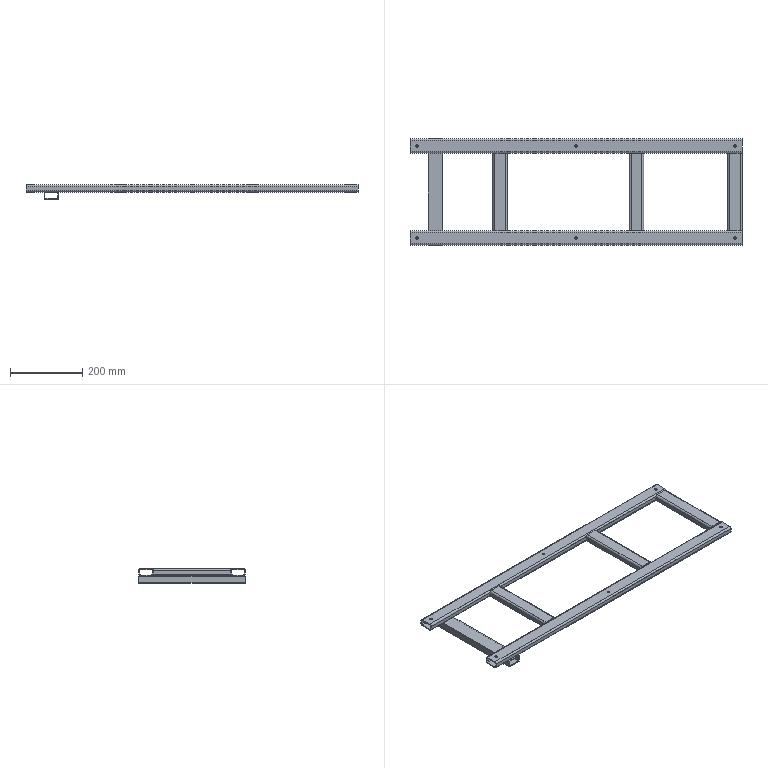Part | SolidWorks | features ICE 2, HoleWzd 1, WeldMemberFeat 1, WeldmentFeature 1 | 6 solids | 136 faces | box 920 x 295 x 40 mm | volume 708311 mm3 | cylinder 64 | plane 60 | cone 12 | commonest cylinder face diameters 7 x24 5 x20 10 x20